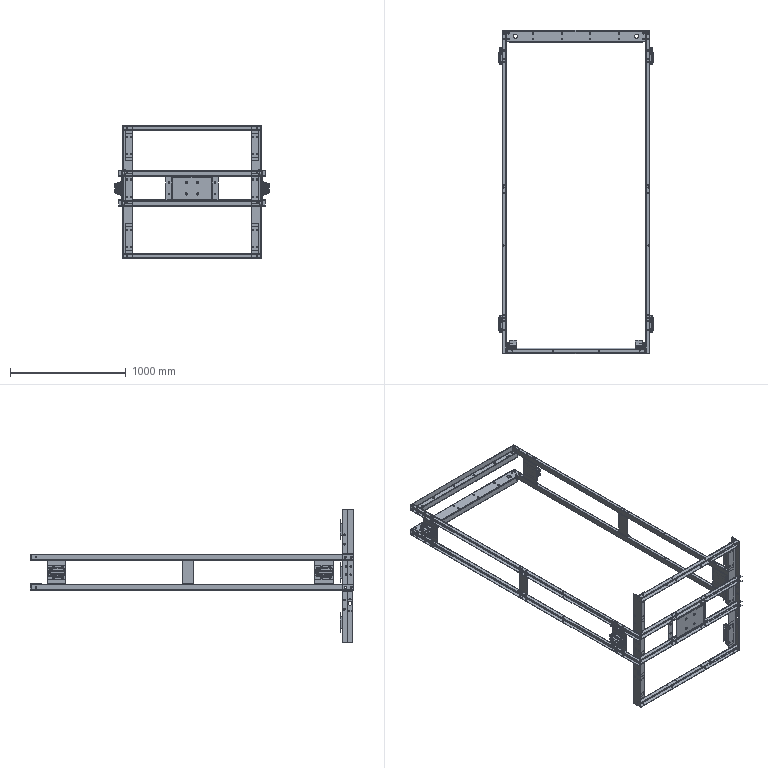Part | SolidWorks | features ReferencePattern 11, MirrorCompFeat 4 | 227 solids | 27522 faces | volume 14365446 mm3 | cylinder 16096 | plane 9226 | cone 2168 | sphere 32 | commonest cylinder face diameters 0.3 x10736 0.4 x2612 6 x820 11 x360 10 x172 4 x136